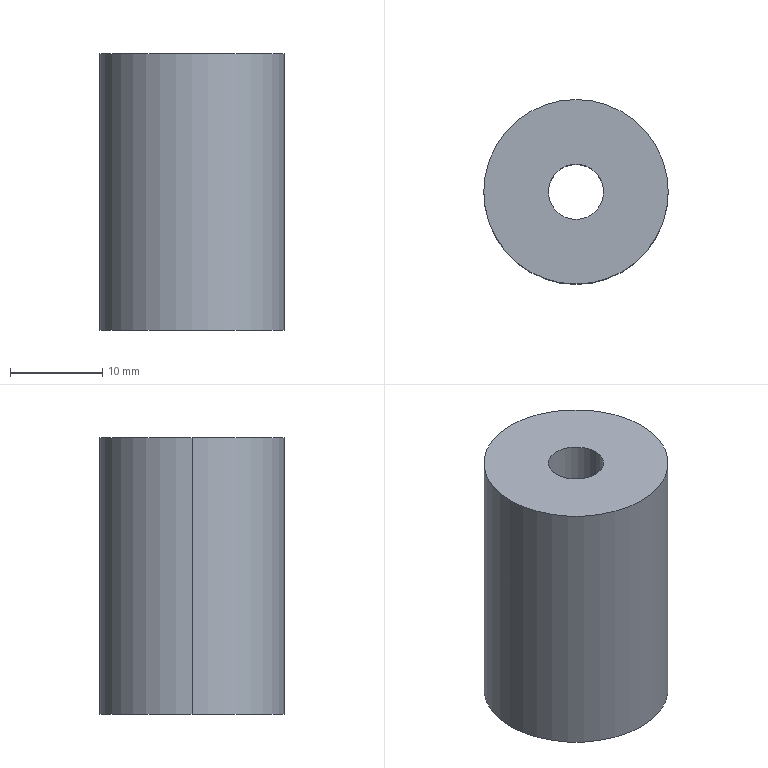Part | STEP file | Polyurethane roller ABA-2030-686-6 | 1 solid | 6 faces | box 20 x 20 x 30 mm | volume 8577 mm3 | cylinder 4 | plane 2 | commonest cylinder face diameters 6 x2 20 x2
STEP:
#1=CARTESIAN_POINT('',(0.,0.,0.));
#2=DIRECTION('',(0.,0.,1.));
#3=DIRECTION('',(1.,0.,0.));
#4=AXIS2_PLACEMENT_3D('',#1,#2,#3);
#5=CARTESIAN_POINT('',(-3.,0.,15.));
#6=VERTEX_POINT('',#5);
#7=CARTESIAN_POINT('',(-3.,0.,-15.));
#8=VERTEX_POINT('',#7);
#9=CARTESIAN_POINT('',(-3.,0.,15.));
#10=DIRECTION('',(0.,0.,-1.));
#11=VECTOR('',#10,1.);
#12=LINE('',#9,#11);
#13=CARTESIAN_POINT('',(0.,0.,15.));
#14=DIRECTION('',(0.,0.,-1.));
#15=DIRECTION('',(-1.,0.,0.));
#16=AXIS2_PLACEMENT_3D('',#13,#14,#15);
#17=CYLINDRICAL_SURFACE('',#16,3.);
#18=CARTESIAN_POINT('',(6.283,0.));
#19=DIRECTION('',(0.,1.));
#20=VECTOR('',#19,1.);
#21=LINE('',#18,#20);
#22=(GEOMETRIC_REPRESENTATION_CONTEXT(2)PARAMETRIC_REPRESENTATION_CONTEXT()REPRESENTATION_CONTEXT('',''));
#23=DEFINITIONAL_REPRESENTATION('',(#21),#22);
#24=PCURVE('',#17,#23);
#25=CARTESIAN_POINT('',(0.,0.,15.));
#26=DIRECTION('',(0.,0.,-1.));
#27=DIRECTION('',(-1.,0.,0.));
#28=AXIS2_PLACEMENT_3D('',#25,#26,#27);
#29=CYLINDRICAL_SURFACE('',#28,3.);
#30=CARTESIAN_POINT('',(0.,0.));
#31=DIRECTION('',(0.,1.));
#32=VECTOR('',#31,1.);
#33=LINE('',#30,#32);
#34=(GEOMETRIC_REPRESENTATION_CONTEXT(2)PARAMETRIC_REPRESENTATION_CONTEXT()REPRESENTATION_CONTEXT('',''));
#35=DEFINITIONAL_REPRESENTATION('',(#33),#34);
#36=PCURVE('',#29,#35);
#37=SURFACE_CURVE('',#12,(#24,#36),.PCURVE_S1.);
#38=EDGE_CURVE('',#6,#8,#37,.T.);
#39=ORIENTED_EDGE('',*,*,#38,.T.);
#40=CARTESIAN_POINT('',(3.,0.,-15.));
#41=VERTEX_POINT('',#40);
#42=CARTESIAN_POINT('',(0.,0.,-15.));
#43=DIRECTION('',(0.,0.,1.));
#44=DIRECTION('',(1.,0.,0.));
#45=AXIS2_PLACEMENT_3D('',#42,#43,#44);
#46=CIRCLE('',#45,3.);
#47=CARTESIAN_POINT('',(9.425,30.));
#48=DIRECTION('',(-1.,0.));
#49=VECTOR('',#48,1.);
#50=LINE('',#47,#49);
#51=(GEOMETRIC_REPRESENTATION_CONTEXT(2)PARAMETRIC_REPRESENTATION_CONTEXT()REPRESENTATION_CONTEXT('',''));
#52=DEFINITIONAL_REPRESENTATION('',(#50),#51);
#53=PCURVE('',#17,#52);
#54=CARTESIAN_POINT('',(0.,0.,-15.));
#55=DIRECTION('',(0.,0.,1.));
#56=DIRECTION('',(1.,0.,0.));
#57=AXIS2_PLACEMENT_3D('',#54,#55,#56);
#58=PLANE('',#57);
#59=CARTESIAN_POINT('',(0.,0.));
#60=DIRECTION('',(1.,0.));
#61=AXIS2_PLACEMENT_2D('',#59,#60);
#62=CIRCLE('',#61,3.);
#63=(GEOMETRIC_REPRESENTATION_CONTEXT(2)PARAMETRIC_REPRESENTATION_CONTEXT()REPRESENTATION_CONTEXT('',''));
#64=DEFINITIONAL_REPRESENTATION('',(#62),#63);
#65=PCURVE('',#58,#64);
#66=SURFACE_CURVE('',#46,(#53,#65),.PCURVE_S1.);
#67=EDGE_CURVE('',#8,#41,#66,.T.);
#68=ORIENTED_EDGE('',*,*,#67,.T.);
#69=CARTESIAN_POINT('',(3.,0.,15.));
#70=VERTEX_POINT('',#69);
#71=CARTESIAN_POINT('',(3.,0.,15.));
#72=DIRECTION('',(0.,0.,-1.));
#73=VECTOR('',#72,1.);
#74=LINE('',#71,#73);
#75=CARTESIAN_POINT('',(3.142,0.));
#76=DIRECTION('',(0.,1.));
#77=VECTOR('',#76,1.);
#78=LINE('',#75,#77);
#79=(GEOMETRIC_REPRESENTATION_CONTEXT(2)PARAMETRIC_REPRESENTATION_CONTEXT()REPRESENTATION_CONTEXT('',''));
#80=DEFINITIONAL_REPRESENTATION('',(#78),#79);
#81=PCURVE('',#17,#80);
#82=CARTESIAN_POINT('',(3.142,0.));
#83=DIRECTION('',(0.,1.));
#84=VECTOR('',#83,1.);
#85=LINE('',#82,#84);
#86=(GEOMETRIC_REPRESENTATION_CONTEXT(2)PARAMETRIC_REPRESENTATION_CONTEXT()REPRESENTATION_CONTEXT('',''));
#87=DEFINITIONAL_REPRESENTATION('',(#85),#86);
#88=PCURVE('',#29,#87);
#89=SURFACE_CURVE('',#74,(#81,#88),.PCURVE_S1.);
#90=EDGE_CURVE('',#70,#41,#89,.T.);
#91=ORIENTED_EDGE('',*,*,#90,.F.);
#92=CARTESIAN_POINT('',(0.,0.,15.));
#93=DIRECTION('',(0.,0.,1.));
#94=DIRECTION('',(1.,0.,0.));
#95=AXIS2_PLACEMENT_3D('',#92,#93,#94);
#96=CIRCLE('',#95,3.);
#97=CARTESIAN_POINT('',(9.425,0.));
#98=DIRECTION('',(-1.,0.));
#99=VECTOR('',#98,1.);
#100=LINE('',#97,#99);
#101=(GEOMETRIC_REPRESENTATION_CONTEXT(2)PARAMETRIC_REPRESENTATION_CONTEXT()REPRESENTATION_CONTEXT('',''));
#102=DEFINITIONAL_REPRESENTATION('',(#100),#101);
#103=PCURVE('',#17,#102);
#104=CARTESIAN_POINT('',(0.,0.,15.));
#105=DIRECTION('',(0.,0.,1.));
#106=DIRECTION('',(1.,0.,0.));
#107=AXIS2_PLACEMENT_3D('',#104,#105,#106);
#108=PLANE('',#107);
#109=CARTESIAN_POINT('',(0.,0.));
#110=DIRECTION('',(1.,0.));
#111=AXIS2_PLACEMENT_2D('',#109,#110);
#112=CIRCLE('',#111,3.);
#113=(GEOMETRIC_REPRESENTATION_CONTEXT(2)PARAMETRIC_REPRESENTATION_CONTEXT()REPRESENTATION_CONTEXT('',''));
#114=DEFINITIONAL_REPRESENTATION('',(#112),#113);
#115=PCURVE('',#108,#114);
#116=SURFACE_CURVE('',#96,(#103,#115),.PCURVE_S1.);
#117=EDGE_CURVE('',#6,#70,#116,.T.);
#118=ORIENTED_EDGE('',*,*,#117,.F.);
#119=EDGE_LOOP('',(#39,#68,#91,#118));
#120=FACE_BOUND('',#119,.F.);
#121=ADVANCED_FACE('',(#120),#17,.F.);
#122=CARTESIAN_POINT('',(10.,0.,15.));
#123=VERTEX_POINT('',#122);
#124=CARTESIAN_POINT('',(-10.,0.,15.));
#125=VERTEX_POINT('',#124);
#126=CARTESIAN_POINT('',(0.,0.,15.));
#127=DIRECTION('',(0.,0.,1.));
#128=DIRECTION('',(1.,0.,0.));
#129=AXIS2_PLACEMENT_3D('',#126,#127,#128);
#130=CIRCLE('',#129,10.);
#131=CARTESIAN_POINT('',(0.,0.,15.));
#132=DIRECTION('',(0.,0.,-1.));
#133=DIRECTION('',(-1.,0.,0.));
#134=AXIS2_PLACEMENT_3D('',#131,#132,#133);
#135=CYLINDRICAL_SURFACE('',#134,10.);
#136=CARTESIAN_POINT('',(3.142,0.));
#137=DIRECTION('',(-1.,0.));
#138=VECTOR('',#137,1.);
#139=LINE('',#136,#138);
#140=(GEOMETRIC_REPRESENTATION_CONTEXT(2)PARAMETRIC_REPRESENTATION_CONTEXT()REPRESENTATION_CONTEXT('',''));
#141=DEFINITIONAL_REPRESENTATION('',(#139),#140);
#142=PCURVE('',#135,#141);
#143=CARTESIAN_POINT('',(0.,0.));
#144=DIRECTION('',(1.,0.));
#145=AXIS2_PLACEMENT_2D('',#143,#144);
#146=CIRCLE('',#145,10.);
#147=(GEOMETRIC_REPRESENTATION_CONTEXT(2)PARAMETRIC_REPRESENTATION_CONTEXT()REPRESENTATION_CONTEXT('',''));
#148=DEFINITIONAL_REPRESENTATION('',(#146),#147);
#149=PCURVE('',#108,#148);
#150=SURFACE_CURVE('',#130,(#142,#149),.PCURVE_S1.);
#151=EDGE_CURVE('',#123,#125,#150,.T.);
#152=ORIENTED_EDGE('',*,*,#151,.F.);
#153=CARTESIAN_POINT('',(10.,0.,-15.));
#154=VERTEX_POINT('',#153);
#155=CARTESIAN_POINT('',(10.,0.,15.));
#156=DIRECTION('',(0.,0.,-1.));
#157=VECTOR('',#156,1.);
#158=LINE('',#155,#157);
#159=CARTESIAN_POINT('',(3.142,0.));
#160=DIRECTION('',(0.,1.));
#161=VECTOR('',#160,1.);
#162=LINE('',#159,#161);
#163=(GEOMETRIC_REPRESENTATION_CONTEXT(2)PARAMETRIC_REPRESENTATION_CONTEXT()REPRESENTATION_CONTEXT('',''));
#164=DEFINITIONAL_REPRESENTATION('',(#162),#163);
#165=PCURVE('',#135,#164);
#166=CARTESIAN_POINT('',(0.,0.,15.));
#167=DIRECTION('',(0.,0.,-1.));
#168=DIRECTION('',(-1.,0.,0.));
#169=AXIS2_PLACEMENT_3D('',#166,#167,#168);
#170=CYLINDRICAL_SURFACE('',#169,10.);
#171=CARTESIAN_POINT('',(3.142,0.));
#172=DIRECTION('',(0.,1.));
#173=VECTOR('',#172,1.);
#174=LINE('',#171,#173);
#175=(GEOMETRIC_REPRESENTATION_CONTEXT(2)PARAMETRIC_REPRESENTATION_CONTEXT()REPRESENTATION_CONTEXT('',''));
#176=DEFINITIONAL_REPRESENTATION('',(#174),#175);
#177=PCURVE('',#170,#176);
#178=SURFACE_CURVE('',#158,(#165,#177),.PCURVE_S1.);
#179=EDGE_CURVE('',#123,#154,#178,.T.);
#180=ORIENTED_EDGE('',*,*,#179,.T.);
#181=CARTESIAN_POINT('',(-10.,0.,-15.));
#182=VERTEX_POINT('',#181);
#183=CARTESIAN_POINT('',(0.,0.,-15.));
#184=DIRECTION('',(0.,0.,1.));
#185=DIRECTION('',(1.,0.,0.));
#186=AXIS2_PLACEMENT_3D('',#183,#184,#185);
#187=CIRCLE('',#186,10.);
#188=CARTESIAN_POINT('',(3.142,30.));
#189=DIRECTION('',(-1.,0.));
#190=VECTOR('',#189,1.);
#191=LINE('',#188,#190);
#192=(GEOMETRIC_REPRESENTATION_CONTEXT(2)PARAMETRIC_REPRESENTATION_CONTEXT()REPRESENTATION_CONTEXT('',''));
#193=DEFINITIONAL_REPRESENTATION('',(#191),#192);
#194=PCURVE('',#135,#193);
#195=CARTESIAN_POINT('',(0.,0.));
#196=DIRECTION('',(1.,0.));
#197=AXIS2_PLACEMENT_2D('',#195,#196);
#198=CIRCLE('',#197,10.);
#199=(GEOMETRIC_REPRESENTATION_CONTEXT(2)PARAMETRIC_REPRESENTATION_CONTEXT()REPRESENTATION_CONTEXT('',''));
#200=DEFINITIONAL_REPRESENTATION('',(#198),#199);
#201=PCURVE('',#58,#200);
#202=SURFACE_CURVE('',#187,(#194,#201),.PCURVE_S1.);
#203=EDGE_CURVE('',#154,#182,#202,.T.);
#204=ORIENTED_EDGE('',*,*,#203,.T.);
#205=CARTESIAN_POINT('',(-10.,0.,15.));
#206=DIRECTION('',(0.,0.,-1.));
#207=VECTOR('',#206,1.);
#208=LINE('',#205,#207);
#209=CARTESIAN_POINT('',(0.,0.));
#210=DIRECTION('',(0.,1.));
#211=VECTOR('',#210,1.);
#212=LINE('',#209,#211);
#213=(GEOMETRIC_REPRESENTATION_CONTEXT(2)PARAMETRIC_REPRESENTATION_CONTEXT()REPRESENTATION_CONTEXT('',''));
#214=DEFINITIONAL_REPRESENTATION('',(#212),#213);
#215=PCURVE('',#135,#214);
#216=CARTESIAN_POINT('',(6.283,0.));
#217=DIRECTION('',(0.,1.));
#218=VECTOR('',#217,1.);
#219=LINE('',#216,#218);
#220=(GEOMETRIC_REPRESENTATION_CONTEXT(2)PARAMETRIC_REPRESENTATION_CONTEXT()REPRESENTATION_CONTEXT('',''));
#221=DEFINITIONAL_REPRESENTATION('',(#219),#220);
#222=PCURVE('',#170,#221);
#223=SURFACE_CURVE('',#208,(#215,#222),.PCURVE_S1.);
#224=EDGE_CURVE('',#125,#182,#223,.T.);
#225=ORIENTED_EDGE('',*,*,#224,.F.);
#226=EDGE_LOOP('',(#152,#180,#204,#225));
#227=FACE_BOUND('',#226,.T.);
#228=ADVANCED_FACE('',(#227),#135,.T.);
#229=CARTESIAN_POINT('',(0.,0.,15.));
#230=DIRECTION('',(0.,0.,1.));
#231=DIRECTION('',(1.,0.,0.));
#232=AXIS2_PLACEMENT_3D('',#229,#230,#231);
#233=CIRCLE('',#232,10.);
#234=CARTESIAN_POINT('',(0.,0.));
#235=DIRECTION('',(1.,0.));
#236=AXIS2_PLACEMENT_2D('',#234,#235);
#237=CIRCLE('',#236,10.);
#238=(GEOMETRIC_REPRESENTATION_CONTEXT(2)PARAMETRIC_REPRESENTATION_CONTEXT()REPRESENTATION_CONTEXT('',''));
#239=DEFINITIONAL_REPRESENTATION('',(#237),#238);
#240=PCURVE('',#108,#239);
#241=CARTESIAN_POINT('',(9.425,0.));
#242=DIRECTION('',(-1.,0.));
#243=VECTOR('',#242,1.);
#244=LINE('',#241,#243);
#245=(GEOMETRIC_REPRESENTATION_CONTEXT(2)PARAMETRIC_REPRESENTATION_CONTEXT()REPRESENTATION_CONTEXT('',''));
#246=DEFINITIONAL_REPRESENTATION('',(#244),#245);
#247=PCURVE('',#170,#246);
#248=SURFACE_CURVE('',#233,(#240,#247),.PCURVE_S1.);
#249=EDGE_CURVE('',#125,#123,#248,.T.);
#250=ORIENTED_EDGE('',*,*,#249,.T.);
#251=ORIENTED_EDGE('',*,*,#151,.T.);
#252=EDGE_LOOP('',(#250,#251));
#253=FACE_BOUND('',#252,.T.);
#254=ORIENTED_EDGE('',*,*,#117,.F.);
#255=CARTESIAN_POINT('',(0.,0.,15.));
#256=DIRECTION('',(0.,0.,1.));
#257=DIRECTION('',(1.,0.,0.));
#258=AXIS2_PLACEMENT_3D('',#255,#256,#257);
#259=CIRCLE('',#258,3.);
#260=CARTESIAN_POINT('',(0.,0.));
#261=DIRECTION('',(1.,0.));
#262=AXIS2_PLACEMENT_2D('',#260,#261);
#263=CIRCLE('',#262,3.);
#264=(GEOMETRIC_REPRESENTATION_CONTEXT(2)PARAMETRIC_REPRESENTATION_CONTEXT()REPRESENTATION_CONTEXT('',''));
#265=DEFINITIONAL_REPRESENTATION('',(#263),#264);
#266=PCURVE('',#108,#265);
#267=CARTESIAN_POINT('',(3.142,0.));
#268=DIRECTION('',(-1.,0.));
#269=VECTOR('',#268,1.);
#270=LINE('',#267,#269);
#271=(GEOMETRIC_REPRESENTATION_CONTEXT(2)PARAMETRIC_REPRESENTATION_CONTEXT()REPRESENTATION_CONTEXT('',''));
#272=DEFINITIONAL_REPRESENTATION('',(#270),#271);
#273=PCURVE('',#29,#272);
#274=SURFACE_CURVE('',#259,(#266,#273),.PCURVE_S1.);
#275=EDGE_CURVE('',#70,#6,#274,.T.);
#276=ORIENTED_EDGE('',*,*,#275,.F.);
#277=EDGE_LOOP('',(#254,#276));
#278=FACE_BOUND('',#277,.T.);
#279=ADVANCED_FACE('',(#253,#278),#108,.T.);
#280=CARTESIAN_POINT('',(0.,0.,-15.));
#281=DIRECTION('',(0.,0.,1.));
#282=DIRECTION('',(1.,0.,0.));
#283=AXIS2_PLACEMENT_3D('',#280,#281,#282);
#284=CIRCLE('',#283,10.);
#285=CARTESIAN_POINT('',(0.,0.));
#286=DIRECTION('',(1.,0.));
#287=AXIS2_PLACEMENT_2D('',#285,#286);
#288=CIRCLE('',#287,10.);
#289=(GEOMETRIC_REPRESENTATION_CONTEXT(2)PARAMETRIC_REPRESENTATION_CONTEXT()REPRESENTATION_CONTEXT('',''));
#290=DEFINITIONAL_REPRESENTATION('',(#288),#289);
#291=PCURVE('',#58,#290);
#292=CARTESIAN_POINT('',(9.425,30.));
#293=DIRECTION('',(-1.,0.));
#294=VECTOR('',#293,1.);
#295=LINE('',#292,#294);
#296=(GEOMETRIC_REPRESENTATION_CONTEXT(2)PARAMETRIC_REPRESENTATION_CONTEXT()REPRESENTATION_CONTEXT('',''));
#297=DEFINITIONAL_REPRESENTATION('',(#295),#296);
#298=PCURVE('',#170,#297);
#299=SURFACE_CURVE('',#284,(#291,#298),.PCURVE_S1.);
#300=EDGE_CURVE('',#182,#154,#299,.T.);
#301=ORIENTED_EDGE('',*,*,#300,.F.);
#302=ORIENTED_EDGE('',*,*,#203,.F.);
#303=EDGE_LOOP('',(#301,#302));
#304=FACE_BOUND('',#303,.T.);
#305=ORIENTED_EDGE('',*,*,#67,.T.);
#306=CARTESIAN_POINT('',(0.,0.,-15.));
#307=DIRECTION('',(0.,0.,1.));
#308=DIRECTION('',(1.,0.,0.));
#309=AXIS2_PLACEMENT_3D('',#306,#307,#308);
#310=CIRCLE('',#309,3.);
#311=CARTESIAN_POINT('',(0.,0.));
#312=DIRECTION('',(1.,0.));
#313=AXIS2_PLACEMENT_2D('',#311,#312);
#314=CIRCLE('',#313,3.);
#315=(GEOMETRIC_REPRESENTATION_CONTEXT(2)PARAMETRIC_REPRESENTATION_CONTEXT()REPRESENTATION_CONTEXT('',''));
#316=DEFINITIONAL_REPRESENTATION('',(#314),#315);
#317=PCURVE('',#58,#316);
#318=CARTESIAN_POINT('',(3.142,30.));
#319=DIRECTION('',(-1.,0.));
#320=VECTOR('',#319,1.);
#321=LINE('',#318,#320);
#322=(GEOMETRIC_REPRESENTATION_CONTEXT(2)PARAMETRIC_REPRESENTATION_CONTEXT()REPRESENTATION_CONTEXT('',''));
#323=DEFINITIONAL_REPRESENTATION('',(#321),#322);
#324=PCURVE('',#29,#323);
#325=SURFACE_CURVE('',#310,(#317,#324),.PCURVE_S1.);
#326=EDGE_CURVE('',#41,#8,#325,.T.);
#327=ORIENTED_EDGE('',*,*,#326,.T.);
#328=EDGE_LOOP('',(#305,#327));
#329=FACE_BOUND('',#328,.T.);
#330=ADVANCED_FACE('',(#304,#329),#58,.F.);
#331=ORIENTED_EDGE('',*,*,#179,.F.);
#332=ORIENTED_EDGE('',*,*,#249,.F.);
#333=ORIENTED_EDGE('',*,*,#224,.T.);
#334=ORIENTED_EDGE('',*,*,#300,.T.);
#335=EDGE_LOOP('',(#331,#332,#333,#334));
#336=FACE_BOUND('',#335,.T.);
#337=ADVANCED_FACE('',(#336),#170,.T.);
#338=ORIENTED_EDGE('',*,*,#326,.T.);
#339=ORIENTED_EDGE('',*,*,#38,.F.);
#340=ORIENTED_EDGE('',*,*,#275,.F.);
#341=ORIENTED_EDGE('',*,*,#90,.T.);
#342=EDGE_LOOP('',(#338,#339,#340,#341));
#343=FACE_BOUND('',#342,.F.);
#344=ADVANCED_FACE('',(#343),#29,.F.);
#345=CLOSED_SHELL('',(#121,#228,#279,#330,#337,#344));
#346=MANIFOLD_SOLID_BREP('',#345);
#347=(LENGTH_UNIT()NAMED_UNIT(*)SI_UNIT(.MILLI.,.METRE.));
#348=UNCERTAINTY_MEASURE_WITH_UNIT(LENGTH_MEASURE(0.0000001),#347,'','');
#349=(NAMED_UNIT(*)PLANE_ANGLE_UNIT()SI_UNIT($,.RADIAN.));
#350=(NAMED_UNIT(*)SI_UNIT($,.STERADIAN.)SOLID_ANGLE_UNIT());
#351=(GEOMETRIC_REPRESENTATION_CONTEXT(3)GLOBAL_UNCERTAINTY_ASSIGNED_CONTEXT((#348))GLOBAL_UNIT_ASSIGNED_CONTEXT((#347,#349,#350))REPRESENTATION_CONTEXT('',''));
#352=ADVANCED_BREP_SHAPE_REPRESENTATION('',(#4,#346),#351);